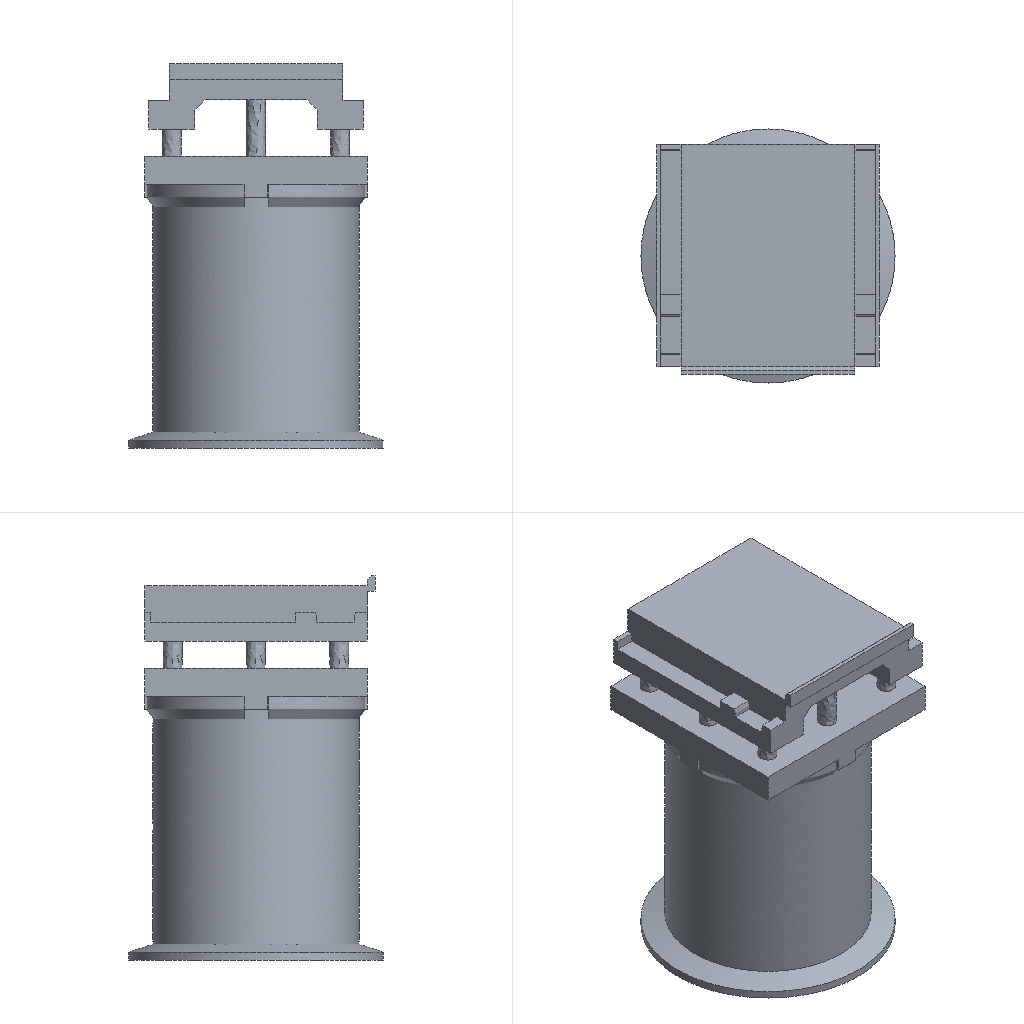Simulation study | ansys workbench
Ansys APDL input file, long lists of numbers shortened:
/batch
/config,noeldb,1     ! force off writing results to database
*get,_wallstrt,active,,time,wall
! ANSYS input file written by Workbench version 2022 R1
! File used for geometry attach:
/title,___--____ 4 (D5)
! ****** Begin Custom Load Command Snippet ******
/COM, ACT Extensions:
/COM,     LSDYNA, 2021.1
/COM,
! ****** End   Custom Load Command Snippet ******
*DIM,_wb_ProjectScratch_dir,string,248
_wb_ProjectScratch_dir(1) = ''
*DIM,_wb_SolverFiles_dir,string,248
_wb_SolverFiles_dir(1) = ''
*DIM,_wb_userfiles_dir,string,248
_wb_userfiles_dir(1) = ''
/com,--- Data in consistent MKS units. See Solving Units in the help system for more information.
/units,MKS
/nopr
/wb,file,start              !  signify a WB generated input file
/prep7
! Turn off shape checking because checks already performed inside WB mesher.
! See help system for more information.
SHPP,OFF,,NOWARN
/nolist
etcon,set             ! allow ANSYS to choose best KEYOP's for 180x elements, resets any applicable keyopt to MAPDL defaults
/com,*********** Nodes for the whole assembly ***********
nblock,3,,165333
(1i9,3e20.9e3)
        1    -4.091861413E+02     3.968814041E+01    -2.039000000E+01
! (150302 more lines like these left out)
-1
/wb,elem,start            !  set before creation of elements
/com,*********** Elements for Body 1 "a953f0-7" ***********
et,1,187
eblock,19,solid,,87505
(19i9)
        1        1        1        1        0        0        0        0       10        0        1    11820    23372    11975    23358    91085    91919    91082    91084
! (175009 more lines like these left out)
-1
/wb,elem,end               !  done creating elements
/com,*********** Send User Defined Coordinate System(s) ***********
csys,0
toffst,273.15,  ! Temperature offset from absolute zero
/com,*********** Set Reference Temperature ***********
tref,22.
/wb,mat,start              !  starting to send materials
/com,*********** Send Materials ***********
Temperature = 'TEMP' ! Temperature
MP,DENS,1,2300,	! kg m^-3
MP,ALPX,1,1.4e-05,	! C^-1
MP,C,1,780,	! J kg^-1 C^-1
MP,KXX,1,0.72,	! W m^-1 C^-1
MP,EX,1,30000000000,	! Pa
MP,NUXY,1,0.18,
/wb,mat,end                !  done sending materials
!************************* Model Summary ********************
!a953f0-7,	混凝土,	matid,	1
!************************* End Model Summary ********************
! get the diagonal of the bounding box. Needed later for other things
*get,_xmin,node,,mnloc,x
*get,_ymin,node,,mnloc,y
*get,_zmin,node,,mnloc,z
*get,_xmax,node,,mxloc,x
*get,_ymax,node,,mxloc,y
*get,_zmax,node,,mxloc,z
_ASMDIAG=(_xmax-_xmin)*(_xmax-_xmin)+(_ymax-_ymin)*(_ymax-_ymin)+(_zmax-_zmin)*(_zmax-_zmin)
_ASMDIAG=SQRT(_ASMDIAG)
/wb,contact,start          !  starting to send contact
/wb,contact,end            !  done creating contacts
/golist
/wb,load,start             !  starting to send loads
/com,*********** Fixed Supports ***********
CMBLOCK,_FIXEDSU,NODE,     7355
(8i10)
         1        96       121       122       123       124       125       126
! (919 more lines like these left out)
cmsel,s,_FIXEDSU
d,all,all
nsel,all
/com,*********** Define Force Using Surface Effect Elements ***********
local,12,0,0.,0.,0.,0.,0.,0.
csys,0
et,2,154
eblock,10,,,7449
(15i9)
   119600        2        2        2       12        4        3     5956     5956    23385    23389     5956    23396
! (7448 more lines like these left out)
-1
esel,s,type,,2
keyop,2,2,1                ! Apply load in local coordinate system
keyop,2,7,1                ! Use original area so load is constant in large deformation
esel,all
/gst,on,on
fini
*get,_numnode,node,0,count
*get,_numelem,elem,0,count
*get, _MAXELEMNUM, elem, 0, NUM, MAX
*get, _MAXNODENUM, node, 0, NUM, MAX
*get, _MAXELEMTYPE, etyp, 0, NUM, MAX
*get, _MAXREALCONST, real, 0, NUM, MAX
/go
/wb,load,end               !  done creating loads
/com,--- Number of total nodes = %_numnode%
/com,--- Number of contact elements = 7449
/com,--- Number of spring elements = 0
/com,--- Number of bearing elements = 0
/com,--- Number of solid elements = 87505
/com,--- Number of condensed parts = 0
/com,--- Number of total elements = %_numelem%
*get,_wallbsol,active,,time,wall
/com,****************************************************************************
/com,*************************    SOLUTION       ********************************
/com,****************************************************************************
/solu
antype,0                   ! static analysis
_thickRatio=  1     ! Ratio of thick parts in the model
eqsl,pcg,1e-8,,,,,,1
cntr,print,1               ! print out contact info and also make no initial contact an error
dmpoption,emat,no             ! Don't combine emat file for DANSYS
dmpoption,esav,no             ! Don't combine esav file for DANSYS
nldiag,cont,iter           ! print out contact info each equilibrium iteration
rescontrol,,none                 ! Do not keep any restart files
/com,****************************************************
/com,******************* SOLVE FOR LS 1 OF 1 ****************
esel,s,type,,2
nsle
sfe,all,1,pres,1,0.
sfe,all,2,pres,1,-1934.784
sfe,all,3,pres,1,0.
nsel,all
esel,all
acel,0.,0.,9.807
/nopr
/gopr
nsub,1,1,1
time,1.
outres,erase
outres,all,none
outres,nsol,all,
outres,rsol,all
outres,eangl,all
outres,etmp,all
outres,veng,all
outres,strs,all,
outres,epel,all,
outres,eppl,all,
outres,cont,all,
! *********** WB SOLVE COMMAND ***********
! check interactive state
*get,ANSINTER_,active,,int
*if,ANSINTER_,ne,0,then
/eof
*endif
solve
/com *************** Write FE CONNECTORS *********
CEWRITE,file,ce,,INTE
/com,****************************************************
/com,*************** FINISHED SOLVE FOR LS 1 *************
*get,_wallasol,active,,time,wall
/nopr
*get,_numnode,node,0,count
*get,_numelem,elem,0,count
*get, _MAXELEMNUM, elem, 0, NUM, MAX
*get, _MAXNODENUM, node, 0, NUM, MAX,,,INTERNAL
*get, _MAXELEMTYPE, etyp, 0, NUM, MAX
*get, _MAXREALCONST, real, 0, NUM, MAX
/gopr
*get,_PCGITER,active,,solu,cgiter
/post1
xmlo,ENCODING,ISO-8859-1
xmlo,parm
/xml,parm,xml
fini
/gopr
*get,_walldone,active,,time,wall
_preptime=(_wallbsol-_wallstrt)*3600
_solvtime=(_wallasol-_wallbsol)*3600
_posttime=(_walldone-_wallasol)*3600
_totaltim=(_walldone-_wallstrt)*3600
*get,_dlbratio,active,0,solu,dlbr
*get,_combtime,active,0,solu,comb
*get,_ssmode,active,0,solu,ssmm
*get,_ndofs,active,0,solu,ndof
*get,_sol_end_time,active,0,set,time
*if,_sol_end_time,eq,1.,then
/fclean				!clean distributed files
*endif
/com,--- Total number of nodes = %_numnode%
/com,--- Total number of elements = %_numelem%
/com,--- Element load balance ratio = %_dlbratio%
/com,--- Time to combine distributed files = %_combtime%
/com,--- Sparse memory mode = %_ssmode%
/com,--- Number of DOF = %_ndofs%
/wb,file,end               ! done with WB generated input